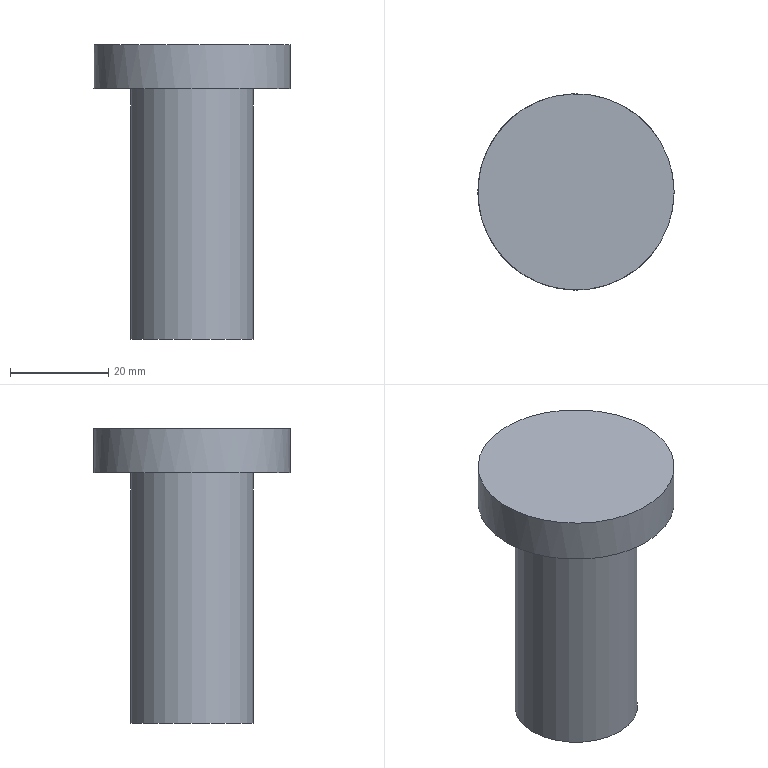Part | NX | features LB-6 2 | 1 solid | 5 faces | box 40 x 40 x 60 mm | volume 36344 mm3 | plane 3 | cylinder 2 | commonest cylinder face diameters 25 x1 40 x1
STEP:
#1=CARTESIAN_POINT('',(3027.766,-906.707,752.716));
#2=VERTEX_POINT('',#1);
#3=CARTESIAN_POINT('',(3040.266,-906.707,752.716));
#4=DIRECTION('',(0.,0.,-1.));
#5=DIRECTION('',(-1.,0.,0.));
#6=AXIS2_PLACEMENT_3D('',#3,#4,#5);
#7=CIRCLE('',#6,12.5);
#8=EDGE_CURVE('',#2,#2,#7,.F.);
#9=ORIENTED_EDGE('',*,*,#8,.F.);
#10=EDGE_LOOP('',(#9));
#11=FACE_BOUND('',#10,.T.);
#12=CARTESIAN_POINT('',(3040.266,-906.707,752.716));
#13=DIRECTION('',(0.,0.,-1.));
#14=DIRECTION('',(-1.,0.,0.));
#15=AXIS2_PLACEMENT_3D('',#12,#13,#14);
#16=PLANE('',#15);
#17=ADVANCED_FACE('',(#11),#16,.T.);
#18=CARTESIAN_POINT('',(3027.766,-906.707,803.716));
#19=VERTEX_POINT('',#18);
#20=CARTESIAN_POINT('',(3040.266,-906.707,803.716));
#21=DIRECTION('',(0.,0.,-1.));
#22=DIRECTION('',(-1.,0.,0.));
#23=AXIS2_PLACEMENT_3D('',#20,#21,#22);
#24=CIRCLE('',#23,12.5);
#25=EDGE_CURVE('',#19,#19,#24,.T.);
#26=ORIENTED_EDGE('',*,*,#25,.T.);
#27=EDGE_LOOP('',(#26));
#28=FACE_BOUND('',#27,.T.);
#29=ORIENTED_EDGE('',*,*,#8,.T.);
#30=EDGE_LOOP('',(#29));
#31=FACE_BOUND('',#30,.T.);
#32=CARTESIAN_POINT('',(3040.266,-906.707,812.716));
#33=DIRECTION('',(0.,0.,-1.));
#34=DIRECTION('',(1.,0.,0.));
#35=AXIS2_PLACEMENT_3D('',#32,#33,#34);
#36=CYLINDRICAL_SURFACE('',#35,12.5);
#37=ADVANCED_FACE('',(#28,#31),#36,.T.);
#38=ORIENTED_EDGE('',*,*,#25,.F.);
#39=EDGE_LOOP('',(#38));
#40=FACE_BOUND('',#39,.T.);
#41=CARTESIAN_POINT('',(3020.266,-906.707,803.716));
#42=VERTEX_POINT('',#41);
#43=CARTESIAN_POINT('',(3040.266,-906.707,803.716));
#44=DIRECTION('',(0.,0.,-1.));
#45=DIRECTION('',(-1.,0.,0.));
#46=AXIS2_PLACEMENT_3D('',#43,#44,#45);
#47=CIRCLE('',#46,20.);
#48=EDGE_CURVE('',#42,#42,#47,.F.);
#49=ORIENTED_EDGE('',*,*,#48,.F.);
#50=EDGE_LOOP('',(#49));
#51=FACE_BOUND('',#50,.T.);
#52=CARTESIAN_POINT('',(3160.094,-859.122,803.716));
#53=DIRECTION('',(0.,0.,-1.));
#54=DIRECTION('',(-1.,0.,0.));
#55=AXIS2_PLACEMENT_3D('',#52,#53,#54);
#56=PLANE('',#55);
#57=ADVANCED_FACE('',(#40,#51),#56,.T.);
#58=CARTESIAN_POINT('',(3060.266,-906.707,812.716));
#59=VERTEX_POINT('',#58);
#60=CARTESIAN_POINT('',(3040.266,-906.707,812.716));
#61=DIRECTION('',(0.,0.,1.));
#62=DIRECTION('',(1.,0.,0.));
#63=AXIS2_PLACEMENT_3D('',#60,#61,#62);
#64=CIRCLE('',#63,20.);
#65=EDGE_CURVE('',#59,#59,#64,.F.);
#66=ORIENTED_EDGE('',*,*,#65,.F.);
#67=EDGE_LOOP('',(#66));
#68=FACE_BOUND('',#67,.T.);
#69=CARTESIAN_POINT('',(3040.266,-906.707,812.716));
#70=DIRECTION('',(0.,0.,1.));
#71=DIRECTION('',(1.,0.,0.));
#72=AXIS2_PLACEMENT_3D('',#69,#70,#71);
#73=PLANE('',#72);
#74=ADVANCED_FACE('',(#68),#73,.T.);
#75=ORIENTED_EDGE('',*,*,#65,.T.);
#76=EDGE_LOOP('',(#75));
#77=FACE_BOUND('',#76,.T.);
#78=ORIENTED_EDGE('',*,*,#48,.T.);
#79=EDGE_LOOP('',(#78));
#80=FACE_BOUND('',#79,.T.);
#81=CARTESIAN_POINT('',(3040.266,-906.707,812.716));
#82=DIRECTION('',(0.,0.,-1.));
#83=DIRECTION('',(1.,0.,0.));
#84=AXIS2_PLACEMENT_3D('',#81,#82,#83);
#85=CYLINDRICAL_SURFACE('',#84,20.);
#86=ADVANCED_FACE('',(#77,#80),#85,.T.);
#87=CLOSED_SHELL('',(#17,#37,#57,#74,#86));
#88=MANIFOLD_SOLID_BREP('',#87);
#89=(LENGTH_UNIT()NAMED_UNIT(*)SI_UNIT(.MILLI.,.METRE.));
#90=UNCERTAINTY_MEASURE_WITH_UNIT(LENGTH_MEASURE(0.00001),#89,'','');
#91=(NAMED_UNIT(*)PLANE_ANGLE_UNIT()SI_UNIT($,.RADIAN.));
#92=(NAMED_UNIT(*)SI_UNIT($,.STERADIAN.)SOLID_ANGLE_UNIT());
#93=(GEOMETRIC_REPRESENTATION_CONTEXT(3)GLOBAL_UNCERTAINTY_ASSIGNED_CONTEXT((#90))GLOBAL_UNIT_ASSIGNED_CONTEXT((#89,#91,#92))REPRESENTATION_CONTEXT('',''));
#94=ADVANCED_BREP_SHAPE_REPRESENTATION('',(#88),#93);